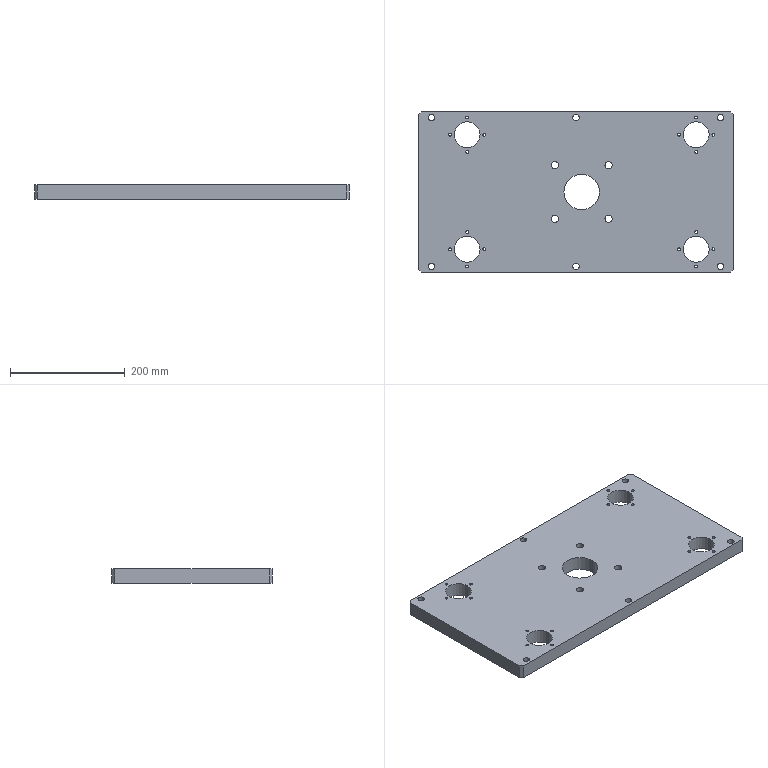Part | STEP file | Lifting Base Plate | 1 solid | 72 faces | box 550 x 280 x 25 mm | volume 3578848 mm3 | cylinder 62 | plane 10 | commonest cylinder face diameters 5 x32 11 x12 13 x8 45 x8 62 x2